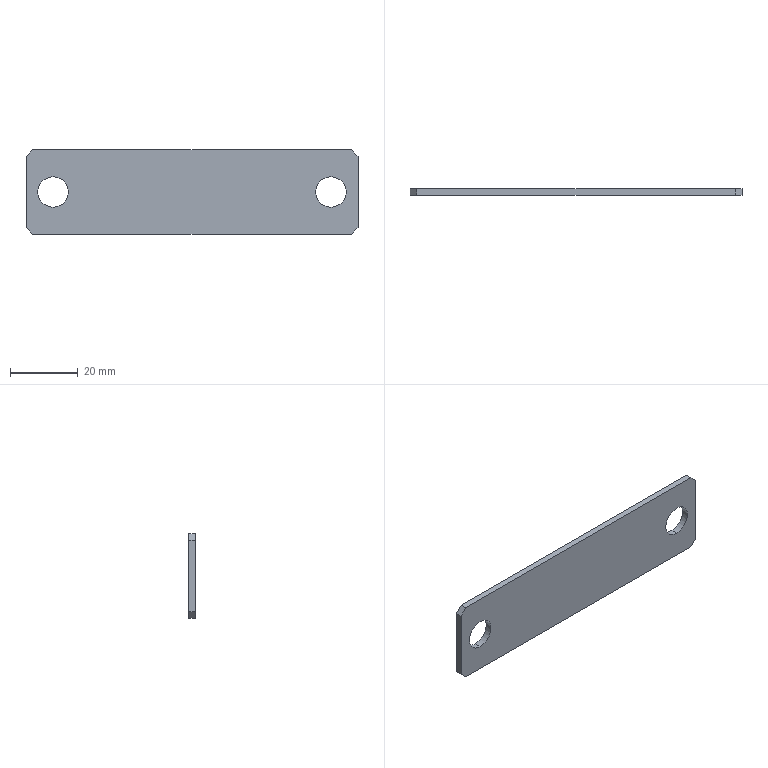Part | STEP file | Vibration plate 3-07_default | 1 solid | 14 faces | box 98 x 2 x 25 mm | volume 4630 mm3 | plane 10 | cylinder 4 | commonest cylinder face diameters 9 x4
STEP:
#1=CARTESIAN_POINT('',(0.,0.,0.));
#2=DIRECTION('',(0.,0.,1.));
#3=DIRECTION('',(1.,0.,0.));
#4=AXIS2_PLACEMENT_3D('',#1,#2,#3);
#5=CARTESIAN_POINT('',(41.,0.,4.5));
#6=VERTEX_POINT('',#5);
#7=CARTESIAN_POINT('',(41.,2.,4.5));
#8=VERTEX_POINT('',#7);
#9=CARTESIAN_POINT('',(41.,2.,4.5));
#10=DIRECTION('',(0.,1.,0.));
#11=VECTOR('',#10,1.);
#12=LINE('',#9,#11);
#13=CARTESIAN_POINT('',(41.,2.,0.));
#14=DIRECTION('',(0.,1.,0.));
#15=DIRECTION('',(0.,0.,1.));
#16=AXIS2_PLACEMENT_3D('',#13,#14,#15);
#17=CYLINDRICAL_SURFACE('',#16,4.5);
#18=CARTESIAN_POINT('',(6.283,0.));
#19=DIRECTION('',(0.,1.));
#20=VECTOR('',#19,1.);
#21=LINE('',#18,#20);
#22=(GEOMETRIC_REPRESENTATION_CONTEXT(2)PARAMETRIC_REPRESENTATION_CONTEXT()REPRESENTATION_CONTEXT('',''));
#23=DEFINITIONAL_REPRESENTATION('',(#21),#22);
#24=PCURVE('',#17,#23);
#25=CARTESIAN_POINT('',(41.,2.,0.));
#26=DIRECTION('',(0.,1.,0.));
#27=DIRECTION('',(0.,0.,1.));
#28=AXIS2_PLACEMENT_3D('',#25,#26,#27);
#29=CYLINDRICAL_SURFACE('',#28,4.5);
#30=CARTESIAN_POINT('',(0.,0.));
#31=DIRECTION('',(0.,1.));
#32=VECTOR('',#31,1.);
#33=LINE('',#30,#32);
#34=(GEOMETRIC_REPRESENTATION_CONTEXT(2)PARAMETRIC_REPRESENTATION_CONTEXT()REPRESENTATION_CONTEXT('',''));
#35=DEFINITIONAL_REPRESENTATION('',(#33),#34);
#36=PCURVE('',#29,#35);
#37=SURFACE_CURVE('',#12,(#24,#36),.PCURVE_S1.);
#38=EDGE_CURVE('',#6,#8,#37,.T.);
#39=ORIENTED_EDGE('',*,*,#38,.T.);
#40=CARTESIAN_POINT('',(41.,2.,-4.5));
#41=VERTEX_POINT('',#40);
#42=CARTESIAN_POINT('',(41.,2.,0.));
#43=DIRECTION('',(0.,-1.,0.));
#44=DIRECTION('',(0.,0.,1.));
#45=AXIS2_PLACEMENT_3D('',#42,#43,#44);
#46=CIRCLE('',#45,4.5);
#47=CARTESIAN_POINT('',(6.283,0.));
#48=DIRECTION('',(-1.,0.));
#49=VECTOR('',#48,1.);
#50=LINE('',#47,#49);
#51=(GEOMETRIC_REPRESENTATION_CONTEXT(2)PARAMETRIC_REPRESENTATION_CONTEXT()REPRESENTATION_CONTEXT('',''));
#52=DEFINITIONAL_REPRESENTATION('',(#50),#51);
#53=PCURVE('',#17,#52);
#54=CARTESIAN_POINT('',(0.,2.,0.));
#55=DIRECTION('',(0.,1.,0.));
#56=DIRECTION('',(0.,0.,1.));
#57=AXIS2_PLACEMENT_3D('',#54,#55,#56);
#58=PLANE('',#57);
#59=CARTESIAN_POINT('',(4.5,41.));
#60=CARTESIAN_POINT('',(4.5,33.206));
#61=CARTESIAN_POINT('',(-2.25,37.103));
#62=CARTESIAN_POINT('',(-9.,41.));
#63=CARTESIAN_POINT('',(-2.25,44.897));
#64=CARTESIAN_POINT('',(4.5,48.794));
#65=CARTESIAN_POINT('',(4.5,41.));
#66=(BOUNDED_CURVE()B_SPLINE_CURVE(2,(#59,#60,#61,#62,#63,#64,#65),.UNSPECIFIED.,.T.,.F.)B_SPLINE_CURVE_WITH_KNOTS((1,2,2,2,2,1),(-2.094,0.,2.094,4.189,6.283,8.378),.UNSPECIFIED.)CURVE()GEOMETRIC_REPRESENTATION_ITEM()RATIONAL_B_SPLINE_CURVE((1.,0.5,1.,0.5,1.,0.5,1.))REPRESENTATION_ITEM(''));
#67=(GEOMETRIC_REPRESENTATION_CONTEXT(2)PARAMETRIC_REPRESENTATION_CONTEXT()REPRESENTATION_CONTEXT('',''));
#68=DEFINITIONAL_REPRESENTATION('',(#66),#67);
#69=PCURVE('',#58,#68);
#70=SURFACE_CURVE('',#46,(#53,#69),.PCURVE_S1.);
#71=EDGE_CURVE('',#8,#41,#70,.T.);
#72=ORIENTED_EDGE('',*,*,#71,.T.);
#73=CARTESIAN_POINT('',(41.,0.,-4.5));
#74=VERTEX_POINT('',#73);
#75=CARTESIAN_POINT('',(41.,2.,-4.5));
#76=DIRECTION('',(0.,1.,0.));
#77=VECTOR('',#76,1.);
#78=LINE('',#75,#77);
#79=CARTESIAN_POINT('',(3.142,0.));
#80=DIRECTION('',(0.,1.));
#81=VECTOR('',#80,1.);
#82=LINE('',#79,#81);
#83=(GEOMETRIC_REPRESENTATION_CONTEXT(2)PARAMETRIC_REPRESENTATION_CONTEXT()REPRESENTATION_CONTEXT('',''));
#84=DEFINITIONAL_REPRESENTATION('',(#82),#83);
#85=PCURVE('',#17,#84);
#86=CARTESIAN_POINT('',(3.142,0.));
#87=DIRECTION('',(0.,1.));
#88=VECTOR('',#87,1.);
#89=LINE('',#86,#88);
#90=(GEOMETRIC_REPRESENTATION_CONTEXT(2)PARAMETRIC_REPRESENTATION_CONTEXT()REPRESENTATION_CONTEXT('',''));
#91=DEFINITIONAL_REPRESENTATION('',(#89),#90);
#92=PCURVE('',#29,#91);
#93=SURFACE_CURVE('',#78,(#85,#92),.PCURVE_S1.);
#94=EDGE_CURVE('',#74,#41,#93,.T.);
#95=ORIENTED_EDGE('',*,*,#94,.F.);
#96=CARTESIAN_POINT('',(41.,0.,0.));
#97=DIRECTION('',(0.,-1.,0.));
#98=DIRECTION('',(0.,0.,1.));
#99=AXIS2_PLACEMENT_3D('',#96,#97,#98);
#100=CIRCLE('',#99,4.5);
#101=CARTESIAN_POINT('',(6.283,-2.));
#102=DIRECTION('',(-1.,0.));
#103=VECTOR('',#102,1.);
#104=LINE('',#101,#103);
#105=(GEOMETRIC_REPRESENTATION_CONTEXT(2)PARAMETRIC_REPRESENTATION_CONTEXT()REPRESENTATION_CONTEXT('',''));
#106=DEFINITIONAL_REPRESENTATION('',(#104),#105);
#107=PCURVE('',#17,#106);
#108=CARTESIAN_POINT('',(0.,0.,0.));
#109=DIRECTION('',(0.,1.,0.));
#110=DIRECTION('',(0.,0.,1.));
#111=AXIS2_PLACEMENT_3D('',#108,#109,#110);
#112=PLANE('',#111);
#113=CARTESIAN_POINT('',(4.5,41.));
#114=CARTESIAN_POINT('',(4.5,33.206));
#115=CARTESIAN_POINT('',(-2.25,37.103));
#116=CARTESIAN_POINT('',(-9.,41.));
#117=CARTESIAN_POINT('',(-2.25,44.897));
#118=CARTESIAN_POINT('',(4.5,48.794));
#119=CARTESIAN_POINT('',(4.5,41.));
#120=(BOUNDED_CURVE()B_SPLINE_CURVE(2,(#113,#114,#115,#116,#117,#118,#119),.UNSPECIFIED.,.T.,.F.)B_SPLINE_CURVE_WITH_KNOTS((1,2,2,2,2,1),(-2.094,0.,2.094,4.189,6.283,8.378),.UNSPECIFIED.)CURVE()GEOMETRIC_REPRESENTATION_ITEM()RATIONAL_B_SPLINE_CURVE((1.,0.5,1.,0.5,1.,0.5,1.))REPRESENTATION_ITEM(''));
#121=(GEOMETRIC_REPRESENTATION_CONTEXT(2)PARAMETRIC_REPRESENTATION_CONTEXT()REPRESENTATION_CONTEXT('',''));
#122=DEFINITIONAL_REPRESENTATION('',(#120),#121);
#123=PCURVE('',#112,#122);
#124=SURFACE_CURVE('',#100,(#107,#123),.PCURVE_S1.);
#125=EDGE_CURVE('',#6,#74,#124,.T.);
#126=ORIENTED_EDGE('',*,*,#125,.F.);
#127=EDGE_LOOP('',(#39,#72,#95,#126));
#128=FACE_BOUND('',#127,.F.);
#129=ADVANCED_FACE('',(#128),#17,.F.);
#130=CARTESIAN_POINT('',(-41.,0.,4.5));
#131=VERTEX_POINT('',#130);
#132=CARTESIAN_POINT('',(-41.,2.,4.5));
#133=VERTEX_POINT('',#132);
#134=CARTESIAN_POINT('',(-41.,2.,4.5));
#135=DIRECTION('',(0.,1.,0.));
#136=VECTOR('',#135,1.);
#137=LINE('',#134,#136);
#138=CARTESIAN_POINT('',(-41.,2.,0.));
#139=DIRECTION('',(0.,1.,0.));
#140=DIRECTION('',(0.,0.,1.));
#141=AXIS2_PLACEMENT_3D('',#138,#139,#140);
#142=CYLINDRICAL_SURFACE('',#141,4.5);
#143=CARTESIAN_POINT('',(6.283,0.));
#144=DIRECTION('',(0.,1.));
#145=VECTOR('',#144,1.);
#146=LINE('',#143,#145);
#147=(GEOMETRIC_REPRESENTATION_CONTEXT(2)PARAMETRIC_REPRESENTATION_CONTEXT()REPRESENTATION_CONTEXT('',''));
#148=DEFINITIONAL_REPRESENTATION('',(#146),#147);
#149=PCURVE('',#142,#148);
#150=CARTESIAN_POINT('',(-41.,2.,0.));
#151=DIRECTION('',(0.,1.,0.));
#152=DIRECTION('',(0.,0.,1.));
#153=AXIS2_PLACEMENT_3D('',#150,#151,#152);
#154=CYLINDRICAL_SURFACE('',#153,4.5);
#155=CARTESIAN_POINT('',(0.,0.));
#156=DIRECTION('',(0.,1.));
#157=VECTOR('',#156,1.);
#158=LINE('',#155,#157);
#159=(GEOMETRIC_REPRESENTATION_CONTEXT(2)PARAMETRIC_REPRESENTATION_CONTEXT()REPRESENTATION_CONTEXT('',''));
#160=DEFINITIONAL_REPRESENTATION('',(#158),#159);
#161=PCURVE('',#154,#160);
#162=SURFACE_CURVE('',#137,(#149,#161),.PCURVE_S1.);
#163=EDGE_CURVE('',#131,#133,#162,.T.);
#164=ORIENTED_EDGE('',*,*,#163,.T.);
#165=CARTESIAN_POINT('',(-41.,2.,-4.5));
#166=VERTEX_POINT('',#165);
#167=CARTESIAN_POINT('',(-41.,2.,0.));
#168=DIRECTION('',(0.,-1.,0.));
#169=DIRECTION('',(0.,0.,1.));
#170=AXIS2_PLACEMENT_3D('',#167,#168,#169);
#171=CIRCLE('',#170,4.5);
#172=CARTESIAN_POINT('',(6.283,0.));
#173=DIRECTION('',(-1.,0.));
#174=VECTOR('',#173,1.);
#175=LINE('',#172,#174);
#176=(GEOMETRIC_REPRESENTATION_CONTEXT(2)PARAMETRIC_REPRESENTATION_CONTEXT()REPRESENTATION_CONTEXT('',''));
#177=DEFINITIONAL_REPRESENTATION('',(#175),#176);
#178=PCURVE('',#142,#177);
#179=CARTESIAN_POINT('',(4.5,-41.));
#180=CARTESIAN_POINT('',(4.5,-48.794));
#181=CARTESIAN_POINT('',(-2.25,-44.897));
#182=CARTESIAN_POINT('',(-9.,-41.));
#183=CARTESIAN_POINT('',(-2.25,-37.103));
#184=CARTESIAN_POINT('',(4.5,-33.206));
#185=CARTESIAN_POINT('',(4.5,-41.));
#186=(BOUNDED_CURVE()B_SPLINE_CURVE(2,(#179,#180,#181,#182,#183,#184,#185),.UNSPECIFIED.,.T.,.F.)B_SPLINE_CURVE_WITH_KNOTS((1,2,2,2,2,1),(-2.094,0.,2.094,4.189,6.283,8.378),.UNSPECIFIED.)CURVE()GEOMETRIC_REPRESENTATION_ITEM()RATIONAL_B_SPLINE_CURVE((1.,0.5,1.,0.5,1.,0.5,1.))REPRESENTATION_ITEM(''));
#187=(GEOMETRIC_REPRESENTATION_CONTEXT(2)PARAMETRIC_REPRESENTATION_CONTEXT()REPRESENTATION_CONTEXT('',''));
#188=DEFINITIONAL_REPRESENTATION('',(#186),#187);
#189=PCURVE('',#58,#188);
#190=SURFACE_CURVE('',#171,(#178,#189),.PCURVE_S1.);
#191=EDGE_CURVE('',#133,#166,#190,.T.);
#192=ORIENTED_EDGE('',*,*,#191,.T.);
#193=CARTESIAN_POINT('',(-41.,0.,-4.5));
#194=VERTEX_POINT('',#193);
#195=CARTESIAN_POINT('',(-41.,2.,-4.5));
#196=DIRECTION('',(0.,1.,0.));
#197=VECTOR('',#196,1.);
#198=LINE('',#195,#197);
#199=CARTESIAN_POINT('',(3.142,0.));
#200=DIRECTION('',(0.,1.));
#201=VECTOR('',#200,1.);
#202=LINE('',#199,#201);
#203=(GEOMETRIC_REPRESENTATION_CONTEXT(2)PARAMETRIC_REPRESENTATION_CONTEXT()REPRESENTATION_CONTEXT('',''));
#204=DEFINITIONAL_REPRESENTATION('',(#202),#203);
#205=PCURVE('',#142,#204);
#206=CARTESIAN_POINT('',(3.142,0.));
#207=DIRECTION('',(0.,1.));
#208=VECTOR('',#207,1.);
#209=LINE('',#206,#208);
#210=(GEOMETRIC_REPRESENTATION_CONTEXT(2)PARAMETRIC_REPRESENTATION_CONTEXT()REPRESENTATION_CONTEXT('',''));
#211=DEFINITIONAL_REPRESENTATION('',(#209),#210);
#212=PCURVE('',#154,#211);
#213=SURFACE_CURVE('',#198,(#205,#212),.PCURVE_S1.);
#214=EDGE_CURVE('',#194,#166,#213,.T.);
#215=ORIENTED_EDGE('',*,*,#214,.F.);
#216=CARTESIAN_POINT('',(-41.,0.,0.));
#217=DIRECTION('',(0.,-1.,0.));
#218=DIRECTION('',(0.,0.,1.));
#219=AXIS2_PLACEMENT_3D('',#216,#217,#218);
#220=CIRCLE('',#219,4.5);
#221=CARTESIAN_POINT('',(6.283,-2.));
#222=DIRECTION('',(-1.,0.));
#223=VECTOR('',#222,1.);
#224=LINE('',#221,#223);
#225=(GEOMETRIC_REPRESENTATION_CONTEXT(2)PARAMETRIC_REPRESENTATION_CONTEXT()REPRESENTATION_CONTEXT('',''));
#226=DEFINITIONAL_REPRESENTATION('',(#224),#225);
#227=PCURVE('',#142,#226);
#228=CARTESIAN_POINT('',(4.5,-41.));
#229=CARTESIAN_POINT('',(4.5,-48.794));
#230=CARTESIAN_POINT('',(-2.25,-44.897));
#231=CARTESIAN_POINT('',(-9.,-41.));
#232=CARTESIAN_POINT('',(-2.25,-37.103));
#233=CARTESIAN_POINT('',(4.5,-33.206));
#234=CARTESIAN_POINT('',(4.5,-41.));
#235=(BOUNDED_CURVE()B_SPLINE_CURVE(2,(#228,#229,#230,#231,#232,#233,#234),.UNSPECIFIED.,.T.,.F.)B_SPLINE_CURVE_WITH_KNOTS((1,2,2,2,2,1),(-2.094,0.,2.094,4.189,6.283,8.378),.UNSPECIFIED.)CURVE()GEOMETRIC_REPRESENTATION_ITEM()RATIONAL_B_SPLINE_CURVE((1.,0.5,1.,0.5,1.,0.5,1.))REPRESENTATION_ITEM(''));
#236=(GEOMETRIC_REPRESENTATION_CONTEXT(2)PARAMETRIC_REPRESENTATION_CONTEXT()REPRESENTATION_CONTEXT('',''));
#237=DEFINITIONAL_REPRESENTATION('',(#235),#236);
#238=PCURVE('',#112,#237);
#239=SURFACE_CURVE('',#220,(#227,#238),.PCURVE_S1.);
#240=EDGE_CURVE('',#131,#194,#239,.T.);
#241=ORIENTED_EDGE('',*,*,#240,.F.);
#242=EDGE_LOOP('',(#164,#192,#215,#241));
#243=FACE_BOUND('',#242,.F.);
#244=ADVANCED_FACE('',(#243),#142,.F.);
#245=ORIENTED_EDGE('',*,*,#125,.F.);
#246=CARTESIAN_POINT('',(41.,0.,0.));
#247=DIRECTION('',(0.,-1.,0.));
#248=DIRECTION('',(0.,0.,1.));
#249=AXIS2_PLACEMENT_3D('',#246,#247,#248);
#250=CIRCLE('',#249,4.5);
#251=CARTESIAN_POINT('',(4.5,41.));
#252=CARTESIAN_POINT('',(4.5,33.206));
#253=CARTESIAN_POINT('',(-2.25,37.103));
#254=CARTESIAN_POINT('',(-9.,41.));
#255=CARTESIAN_POINT('',(-2.25,44.897));
#256=CARTESIAN_POINT('',(4.5,48.794));
#257=CARTESIAN_POINT('',(4.5,41.));
#258=(BOUNDED_CURVE()B_SPLINE_CURVE(2,(#251,#252,#253,#254,#255,#256,#257),.UNSPECIFIED.,.T.,.F.)B_SPLINE_CURVE_WITH_KNOTS((1,2,2,2,2,1),(-2.094,0.,2.094,4.189,6.283,8.378),.UNSPECIFIED.)CURVE()GEOMETRIC_REPRESENTATION_ITEM()RATIONAL_B_SPLINE_CURVE((1.,0.5,1.,0.5,1.,0.5,1.))REPRESENTATION_ITEM(''));
#259=(GEOMETRIC_REPRESENTATION_CONTEXT(2)PARAMETRIC_REPRESENTATION_CONTEXT()REPRESENTATION_CONTEXT('',''));
#260=DEFINITIONAL_REPRESENTATION('',(#258),#259);
#261=PCURVE('',#112,#260);
#262=CARTESIAN_POINT('',(6.283,-2.));
#263=DIRECTION('',(-1.,0.));
#264=VECTOR('',#263,1.);
#265=LINE('',#262,#264);
#266=(GEOMETRIC_REPRESENTATION_CONTEXT(2)PARAMETRIC_REPRESENTATION_CONTEXT()REPRESENTATION_CONTEXT('',''));
#267=DEFINITIONAL_REPRESENTATION('',(#265),#266);
#268=PCURVE('',#29,#267);
#269=SURFACE_CURVE('',#250,(#261,#268),.PCURVE_S1.);
#270=EDGE_CURVE('',#74,#6,#269,.T.);
#271=ORIENTED_EDGE('',*,*,#270,.F.);
#272=EDGE_LOOP('',(#245,#271));
#273=FACE_BOUND('',#272,.T.);
#274=ORIENTED_EDGE('',*,*,#240,.F.);
#275=CARTESIAN_POINT('',(-41.,0.,0.));
#276=DIRECTION('',(0.,-1.,0.));
#277=DIRECTION('',(0.,0.,1.));
#278=AXIS2_PLACEMENT_3D('',#275,#276,#277);
#279=CIRCLE('',#278,4.5);
#280=CARTESIAN_POINT('',(4.5,-41.));
#281=CARTESIAN_POINT('',(4.5,-48.794));
#282=CARTESIAN_POINT('',(-2.25,-44.897));
#283=CARTESIAN_POINT('',(-9.,-41.));
#284=CARTESIAN_POINT('',(-2.25,-37.103));
#285=CARTESIAN_POINT('',(4.5,-33.206));
#286=CARTESIAN_POINT('',(4.5,-41.));
#287=(BOUNDED_CURVE()B_SPLINE_CURVE(2,(#280,#281,#282,#283,#284,#285,#286),.UNSPECIFIED.,.T.,.F.)B_SPLINE_CURVE_WITH_KNOTS((1,2,2,2,2,1),(-2.094,0.,2.094,4.189,6.283,8.378),.UNSPECIFIED.)CURVE()GEOMETRIC_REPRESENTATION_ITEM()RATIONAL_B_SPLINE_CURVE((1.,0.5,1.,0.5,1.,0.5,1.))REPRESENTATION_ITEM(''));
#288=(GEOMETRIC_REPRESENTATION_CONTEXT(2)PARAMETRIC_REPRESENTATION_CONTEXT()REPRESENTATION_CONTEXT('',''));
#289=DEFINITIONAL_REPRESENTATION('',(#287),#288);
#290=PCURVE('',#112,#289);
#291=CARTESIAN_POINT('',(6.283,-2.));
#292=DIRECTION('',(-1.,0.));
#293=VECTOR('',#292,1.);
#294=LINE('',#291,#293);
#295=(GEOMETRIC_REPRESENTATION_CONTEXT(2)PARAMETRIC_REPRESENTATION_CONTEXT()REPRESENTATION_CONTEXT('',''));
#296=DEFINITIONAL_REPRESENTATION('',(#294),#295);
#297=PCURVE('',#154,#296);
#298=SURFACE_CURVE('',#279,(#290,#297),.PCURVE_S1.);
#299=EDGE_CURVE('',#194,#131,#298,.T.);
#300=ORIENTED_EDGE('',*,*,#299,.F.);
#301=EDGE_LOOP('',(#274,#300));
#302=FACE_BOUND('',#301,.T.);
#303=CARTESIAN_POINT('',(-49.,0.,10.5));
#304=VERTEX_POINT('',#303);
#305=CARTESIAN_POINT('',(-47.,0.,12.5));
#306=VERTEX_POINT('',#305);
#307=CARTESIAN_POINT('',(-49.,0.,10.5));
#308=DIRECTION('',(0.7071,0.,0.7071));
#309=VECTOR('',#308,1.);
#310=LINE('',#307,#309);
#311=CARTESIAN_POINT('',(10.5,-49.));
#312=DIRECTION('',(0.7071,0.7071));
#313=VECTOR('',#312,1.);
#314=LINE('',#311,#313);
#315=(GEOMETRIC_REPRESENTATION_CONTEXT(2)PARAMETRIC_REPRESENTATION_CONTEXT()REPRESENTATION_CONTEXT('',''));
#316=DEFINITIONAL_REPRESENTATION('',(#314),#315);
#317=PCURVE('',#112,#316);
#318=CARTESIAN_POINT('',(-48.,1.,11.5));
#319=DIRECTION('',(-0.7071,0.,0.7071));
#320=DIRECTION('',(0.7071,0.,0.7071));
#321=AXIS2_PLACEMENT_3D('',#318,#319,#320);
#322=PLANE('',#321);
#323=CARTESIAN_POINT('',(-1.414,-1.));
#324=DIRECTION('',(1.,0.));
#325=VECTOR('',#324,1.);
#326=LINE('',#323,#325);
#327=(GEOMETRIC_REPRESENTATION_CONTEXT(2)PARAMETRIC_REPRESENTATION_CONTEXT()REPRESENTATION_CONTEXT('',''));
#328=DEFINITIONAL_REPRESENTATION('',(#326),#327);
#329=PCURVE('',#322,#328);
#330=SURFACE_CURVE('',#310,(#317,#329),.PCURVE_S1.);
#331=EDGE_CURVE('',#304,#306,#330,.T.);
#332=ORIENTED_EDGE('',*,*,#331,.F.);
#333=CARTESIAN_POINT('',(-49.,0.,-10.5));
#334=VERTEX_POINT('',#333);
#335=CARTESIAN_POINT('',(-49.,0.,0.));
#336=DIRECTION('',(0.,0.,1.));
#337=VECTOR('',#336,1.);
#338=LINE('',#335,#337);
#339=CARTESIAN_POINT('',(0.,-49.));
#340=DIRECTION('',(1.,0.));
#341=VECTOR('',#340,1.);
#342=LINE('',#339,#341);
#343=(GEOMETRIC_REPRESENTATION_CONTEXT(2)PARAMETRIC_REPRESENTATION_CONTEXT()REPRESENTATION_CONTEXT('',''));
#344=DEFINITIONAL_REPRESENTATION('',(#342),#343);
#345=PCURVE('',#112,#344);
#346=CARTESIAN_POINT('',(-49.,0.,-12.5));
#347=DIRECTION('',(-1.,0.,0.));
#348=DIRECTION('',(0.,0.,1.));
#349=AXIS2_PLACEMENT_3D('',#346,#347,#348);
#350=PLANE('',#349);
#351=CARTESIAN_POINT('',(12.5,0.));
#352=DIRECTION('',(1.,0.));
#353=VECTOR('',#352,1.);
#354=LINE('',#351,#353);
#355=(GEOMETRIC_REPRESENTATION_CONTEXT(2)PARAMETRIC_REPRESENTATION_CONTEXT()REPRESENTATION_CONTEXT('',''));
#356=DEFINITIONAL_REPRESENTATION('',(#354),#355);
#357=PCURVE('',#350,#356);
#358=SURFACE_CURVE('',#338,(#345,#357),.PCURVE_S1.);
#359=EDGE_CURVE('',#334,#304,#358,.T.);
#360=ORIENTED_EDGE('',*,*,#359,.F.);
#361=CARTESIAN_POINT('',(-47.,0.,-12.5));
#362=VERTEX_POINT('',#361);
#363=CARTESIAN_POINT('',(-47.,0.,-12.5));
#364=DIRECTION('',(-0.7071,0.,0.7071));
#365=VECTOR('',#364,1.);
#366=LINE('',#363,#365);
#367=CARTESIAN_POINT('',(-12.5,-47.));
#368=DIRECTION('',(0.7071,-0.7071));
#369=VECTOR('',#368,1.);
#370=LINE('',#367,#369);
#371=(GEOMETRIC_REPRESENTATION_CONTEXT(2)PARAMETRIC_REPRESENTATION_CONTEXT()REPRESENTATION_CONTEXT('',''));
#372=DEFINITIONAL_REPRESENTATION('',(#370),#371);
#373=PCURVE('',#112,#372);
#374=CARTESIAN_POINT('',(-48.,1.,-11.5));
#375=DIRECTION('',(-0.7071,0.,-0.7071));
#376=DIRECTION('',(-0.7071,0.,0.7071));
#377=AXIS2_PLACEMENT_3D('',#374,#375,#376);
#378=PLANE('',#377);
#379=CARTESIAN_POINT('',(-1.414,-1.));
#380=DIRECTION('',(1.,0.));
#381=VECTOR('',#380,1.);
#382=LINE('',#379,#381);
#383=(GEOMETRIC_REPRESENTATION_CONTEXT(2)PARAMETRIC_REPRESENTATION_CONTEXT()REPRESENTATION_CONTEXT('',''));
#384=DEFINITIONAL_REPRESENTATION('',(#382),#383);
#385=PCURVE('',#378,#384);
#386=SURFACE_CURVE('',#366,(#373,#385),.PCURVE_S1.);
#387=EDGE_CURVE('',#362,#334,#386,.T.);
#388=ORIENTED_EDGE('',*,*,#387,.F.);
#389=CARTESIAN_POINT('',(47.,0.,-12.5));
#390=VERTEX_POINT('',#389);
#391=CARTESIAN_POINT('',(0.,0.,-12.5));
#392=DIRECTION('',(-1.,0.,0.));
#393=VECTOR('',#392,1.);
#394=LINE('',#391,#393);
#395=CARTESIAN_POINT('',(-12.5,0.));
#396=DIRECTION('',(0.,-1.));
#397=VECTOR('',#396,1.);
#398=LINE('',#395,#397);
#399=(GEOMETRIC_REPRESENTATION_CONTEXT(2)PARAMETRIC_REPRESENTATION_CONTEXT()REPRESENTATION_CONTEXT('',''));
#400=DEFINITIONAL_REPRESENTATION('',(#398),#399);
#401=PCURVE('',#112,#400);
#402=CARTESIAN_POINT('',(49.,0.,-12.5));
#403=DIRECTION('',(0.,0.,-1.));
#404=DIRECTION('',(-1.,0.,0.));
#405=AXIS2_PLACEMENT_3D('',#402,#403,#404);
#406=PLANE('',#405);
#407=CARTESIAN_POINT('',(49.,0.));
#408=DIRECTION('',(1.,0.));
#409=VECTOR('',#408,1.);
#410=LINE('',#407,#409);
#411=(GEOMETRIC_REPRESENTATION_CONTEXT(2)PARAMETRIC_REPRESENTATION_CONTEXT()REPRESENTATION_CONTEXT('',''));
#412=DEFINITIONAL_REPRESENTATION('',(#410),#411);
#413=PCURVE('',#406,#412);
#414=SURFACE_CURVE('',#394,(#401,#413),.PCURVE_S1.);
#415=EDGE_CURVE('',#390,#362,#414,.T.);
#416=ORIENTED_EDGE('',*,*,#415,.F.);
#417=CARTESIAN_POINT('',(49.,0.,-10.5));
#418=VERTEX_POINT('',#417);
#419=CARTESIAN_POINT('',(49.,0.,-10.5));
#420=DIRECTION('',(-0.7071,0.,-0.7071));
#421=VECTOR('',#420,1.);
#422=LINE('',#419,#421);
#423=CARTESIAN_POINT('',(-10.5,49.));
#424=DIRECTION('',(-0.7071,-0.7071));
#425=VECTOR('',#424,1.);
#426=LINE('',#423,#425);
#427=(GEOMETRIC_REPRESENTATION_CONTEXT(2)PARAMETRIC_REPRESENTATION_CONTEXT()REPRESENTATION_CONTEXT('',''));
#428=DEFINITIONAL_REPRESENTATION('',(#426),#427);
#429=PCURVE('',#112,#428);
#430=CARTESIAN_POINT('',(48.,1.,-11.5));
#431=DIRECTION('',(0.7071,0.,-0.7071));
#432=DIRECTION('',(-0.7071,0.,-0.7071));
#433=AXIS2_PLACEMENT_3D('',#430,#431,#432);
#434=PLANE('',#433);
#435=CARTESIAN_POINT('',(-1.414,-1.));
#436=DIRECTION('',(1.,0.));
#437=VECTOR('',#436,1.);
#438=LINE('',#435,#437);
#439=(GEOMETRIC_REPRESENTATION_CONTEXT(2)PARAMETRIC_REPRESENTATION_CONTEXT()REPRESENTATION_CONTEXT('',''));
#440=DEFINITIONAL_REPRESENTATION('',(#438),#439);
#441=PCURVE('',#434,#440);
#442=SURFACE_CURVE('',#422,(#429,#441),.PCURVE_S1.);
#443=EDGE_CURVE('',#418,#390,#442,.T.);
#444=ORIENTED_EDGE('',*,*,#443,.F.);
#445=CARTESIAN_POINT('',(49.,0.,10.5));
#446=VERTEX_POINT('',#445);
#447=CARTESIAN_POINT('',(49.,0.,0.));
#448=DIRECTION('',(0.,0.,-1.));
#449=VECTOR('',#448,1.);
#450=LINE('',#447,#449);
#451=CARTESIAN_POINT('',(0.,49.));
#452=DIRECTION('',(-1.,0.));
#453=VECTOR('',#452,1.);
#454=LINE('',#451,#453);
#455=(GEOMETRIC_REPRESENTATION_CONTEXT(2)PARAMETRIC_REPRESENTATION_CONTEXT()REPRESENTATION_CONTEXT('',''));
#456=DEFINITIONAL_REPRESENTATION('',(#454),#455);
#457=PCURVE('',#112,#456);
#458=CARTESIAN_POINT('',(49.,0.,12.5));
#459=DIRECTION('',(1.,0.,0.));
#460=DIRECTION('',(0.,0.,-1.));
#461=AXIS2_PLACEMENT_3D('',#458,#459,#460);
#462=PLANE('',#461);
#463=CARTESIAN_POINT('',(12.5,0.));
#464=DIRECTION('',(1.,0.));
#465=VECTOR('',#464,1.);
#466=LINE('',#463,#465);
#467=(GEOMETRIC_REPRESENTATION_CONTEXT(2)PARAMETRIC_REPRESENTATION_CONTEXT()REPRESENTATION_CONTEXT('',''));
#468=DEFINITIONAL_REPRESENTATION('',(#466),#467);
#469=PCURVE('',#462,#468);
#470=SURFACE_CURVE('',#450,(#457,#469),.PCURVE_S1.);
#471=EDGE_CURVE('',#446,#418,#470,.T.);
#472=ORIENTED_EDGE('',*,*,#471,.F.);
#473=CARTESIAN_POINT('',(47.,0.,12.5));
#474=VERTEX_POINT('',#473);
#475=CARTESIAN_POINT('',(47.,0.,12.5));
#476=DIRECTION('',(0.7071,0.,-0.7071));
#477=VECTOR('',#476,1.);
#478=LINE('',#475,#477);
#479=CARTESIAN_POINT('',(12.5,47.));
#480=DIRECTION('',(-0.7071,0.7071));
#481=VECTOR('',#480,1.);
#482=LINE('',#479,#481);
#483=(GEOMETRIC_REPRESENTATION_CONTEXT(2)PARAMETRIC_REPRESENTATION_CONTEXT()REPRESENTATION_CONTEXT('',''));
#484=DEFINITIONAL_REPRESENTATION('',(#482),#483);
#485=PCURVE('',#112,#484);
#486=CARTESIAN_POINT('',(48.,1.,11.5));
#487=DIRECTION('',(0.7071,0.,0.7071));
#488=DIRECTION('',(0.7071,0.,-0.7071));
#489=AXIS2_PLACEMENT_3D('',#486,#487,#488);
#490=PLANE('',#489);
#491=CARTESIAN_POINT('',(-1.414,-1.));
#492=DIRECTION('',(1.,0.));
#493=VECTOR('',#492,1.);
#494=LINE('',#491,#493);
#495=(GEOMETRIC_REPRESENTATION_CONTEXT(2)PARAMETRIC_REPRESENTATION_CONTEXT()REPRESENTATION_CONTEXT('',''));
#496=DEFINITIONAL_REPRESENTATION('',(#494),#495);
#497=PCURVE('',#490,#496);
#498=SURFACE_CURVE('',#478,(#485,#497),.PCURVE_S1.);
#499=EDGE_CURVE('',#474,#446,#498,.T.);
#500=ORIENTED_EDGE('',*,*,#499,.F.);
#501=CARTESIAN_POINT('',(0.,0.,12.5));
#502=DIRECTION('',(1.,0.,0.));
#503=VECTOR('',#502,1.);
#504=LINE('',#501,#503);
#505=CARTESIAN_POINT('',(12.5,0.));
#506=DIRECTION('',(0.,1.));
#507=VECTOR('',#506,1.);
#508=LINE('',#505,#507);
#509=(GEOMETRIC_REPRESENTATION_CONTEXT(2)PARAMETRIC_REPRESENTATION_CONTEXT()REPRESENTATION_CONTEXT('',''));
#510=DEFINITIONAL_REPRESENTATION('',(#508),#509);
#511=PCURVE('',#112,#510);
#512=CARTESIAN_POINT('',(-49.,0.,12.5));
#513=DIRECTION('',(0.,0.,1.));
#514=DIRECTION('',(1.,0.,0.));
#515=AXIS2_PLACEMENT_3D('',#512,#513,#514);
#516=PLANE('',#515);
#517=CARTESIAN_POINT('',(49.,0.));
#518=DIRECTION('',(1.,0.));
#519=VECTOR('',#518,1.);
#520=LINE('',#517,#519);
#521=(GEOMETRIC_REPRESENTATION_CONTEXT(2)PARAMETRIC_REPRESENTATION_CONTEXT()REPRESENTATION_CONTEXT('',''));
#522=DEFINITIONAL_REPRESENTATION('',(#520),#521);
#523=PCURVE('',#516,#522);
#524=SURFACE_CURVE('',#504,(#511,#523),.PCURVE_S1.);
#525=EDGE_CURVE('',#306,#474,#524,.T.);
#526=ORIENTED_EDGE('',*,*,#525,.F.);
#527=EDGE_LOOP('',(#332,#360,#388,#416,#444,#472,#500,#526));
#528=FACE_BOUND('',#527,.T.);
#529=ADVANCED_FACE('',(#273,#302,#528),#112,.F.);
#530=CARTESIAN_POINT('',(41.,2.,0.));
#531=DIRECTION('',(0.,-1.,0.));
#532=DIRECTION('',(0.,0.,1.));
#533=AXIS2_PLACEMENT_3D('',#530,#531,#532);
#534=CIRCLE('',#533,4.5);
#535=CARTESIAN_POINT('',(6.283,0.));
#536=DIRECTION('',(-1.,0.));
#537=VECTOR('',#536,1.);
#538=LINE('',#535,#537);
#539=(GEOMETRIC_REPRESENTATION_CONTEXT(2)PARAMETRIC_REPRESENTATION_CONTEXT()REPRESENTATION_CONTEXT('',''));
#540=DEFINITIONAL_REPRESENTATION('',(#538),#539);
#541=PCURVE('',#29,#540);
#542=CARTESIAN_POINT('',(4.5,41.));
#543=CARTESIAN_POINT('',(4.5,33.206));
#544=CARTESIAN_POINT('',(-2.25,37.103));
#545=CARTESIAN_POINT('',(-9.,41.));
#546=CARTESIAN_POINT('',(-2.25,44.897));
#547=CARTESIAN_POINT('',(4.5,48.794));
#548=CARTESIAN_POINT('',(4.5,41.));
#549=(BOUNDED_CURVE()B_SPLINE_CURVE(2,(#542,#543,#544,#545,#546,#547,#548),.UNSPECIFIED.,.T.,.F.)B_SPLINE_CURVE_WITH_KNOTS((1,2,2,2,2,1),(-2.094,0.,2.094,4.189,6.283,8.378),.UNSPECIFIED.)CURVE()GEOMETRIC_REPRESENTATION_ITEM()RATIONAL_B_SPLINE_CURVE((1.,0.5,1.,0.5,1.,0.5,1.))REPRESENTATION_ITEM(''));
#550=(GEOMETRIC_REPRESENTATION_CONTEXT(2)PARAMETRIC_REPRESENTATION_CONTEXT()REPRESENTATION_CONTEXT('',''));
#551=DEFINITIONAL_REPRESENTATION('',(#549),#550);
#552=PCURVE('',#58,#551);
#553=SURFACE_CURVE('',#534,(#541,#552),.PCURVE_S1.);
#554=EDGE_CURVE('',#41,#8,#553,.T.);
#555=ORIENTED_EDGE('',*,*,#554,.T.);
#556=ORIENTED_EDGE('',*,*,#38,.F.);
#557=ORIENTED_EDGE('',*,*,#270,.F.);
#558=ORIENTED_EDGE('',*,*,#94,.T.);
#559=EDGE_LOOP('',(#555,#556,#557,#558));
#560=FACE_BOUND('',#559,.F.);
#561=ADVANCED_FACE('',(#560),#29,.F.);
#562=CARTESIAN_POINT('',(-41.,2.,0.));
#563=DIRECTION('',(0.,-1.,0.));
#564=DIRECTION('',(0.,0.,1.));
#565=AXIS2_PLACEMENT_3D('',#562,#563,#564);
#566=CIRCLE('',#565,4.5);
#567=CARTESIAN_POINT('',(6.283,0.));
#568=DIRECTION('',(-1.,0.));
#569=VECTOR('',#568,1.);
#570=LINE('',#567,#569);
#571=(GEOMETRIC_REPRESENTATION_CONTEXT(2)PARAMETRIC_REPRESENTATION_CONTEXT()REPRESENTATION_CONTEXT('',''));
#572=DEFINITIONAL_REPRESENTATION('',(#570),#571);
#573=PCURVE('',#154,#572);
#574=CARTESIAN_POINT('',(4.5,-41.));
#575=CARTESIAN_POINT('',(4.5,-48.794));
#576=CARTESIAN_POINT('',(-2.25,-44.897));
#577=CARTESIAN_POINT('',(-9.,-41.));
#578=CARTESIAN_POINT('',(-2.25,-37.103));
#579=CARTESIAN_POINT('',(4.5,-33.206));
#580=CARTESIAN_POINT('',(4.5,-41.));
#581=(BOUNDED_CURVE()B_SPLINE_CURVE(2,(#574,#575,#576,#577,#578,#579,#580),.UNSPECIFIED.,.T.,.F.)B_SPLINE_CURVE_WITH_KNOTS((1,2,2,2,2,1),(-2.094,0.,2.094,4.189,6.283,8.378),.UNSPECIFIED.)CURVE()GEOMETRIC_REPRESENTATION_ITEM()RATIONAL_B_SPLINE_CURVE((1.,0.5,1.,0.5,1.,0.5,1.))REPRESENTATION_ITEM(''));
#582=(GEOMETRIC_REPRESENTATION_CONTEXT(2)PARAMETRIC_REPRESENTATION_CONTEXT()REPRESENTATION_CONTEXT('',''));
#583=DEFINITIONAL_REPRESENTATION('',(#581),#582);
#584=PCURVE('',#58,#583);
#585=SURFACE_CURVE('',#566,(#573,#584),.PCURVE_S1.);
#586=EDGE_CURVE('',#166,#133,#585,.T.);
#587=ORIENTED_EDGE('',*,*,#586,.T.);
#588=ORIENTED_EDGE('',*,*,#163,.F.);
#589=ORIENTED_EDGE('',*,*,#299,.F.);
#590=ORIENTED_EDGE('',*,*,#214,.T.);
#591=EDGE_LOOP('',(#587,#588,#589,#590));
#592=FACE_BOUND('',#591,.F.);
#593=ADVANCED_FACE('',(#592),#154,.F.);
#594=ORIENTED_EDGE('',*,*,#525,.T.);
#595=CARTESIAN_POINT('',(47.,2.,12.5));
#596=VERTEX_POINT('',#595);
#597=CARTESIAN_POINT('',(47.,0.,12.5));
#598=DIRECTION('',(0.,1.,0.));
#599=VECTOR('',#598,1.);
#600=LINE('',#597,#599);
#601=CARTESIAN_POINT('',(96.,0.));
#602=DIRECTION('',(0.,1.));
#603=VECTOR('',#602,1.);
#604=LINE('',#601,#603);
#605=(GEOMETRIC_REPRESENTATION_CONTEXT(2)PARAMETRIC_REPRESENTATION_CONTEXT()REPRESENTATION_CONTEXT('',''));
#606=DEFINITIONAL_REPRESENTATION('',(#604),#605);
#607=PCURVE('',#516,#606);
#608=CARTESIAN_POINT('',(-1.414,-1.));
#609=DIRECTION('',(0.,1.));
#610=VECTOR('',#609,1.);
#611=LINE('',#608,#610);
#612=(GEOMETRIC_REPRESENTATION_CONTEXT(2)PARAMETRIC_REPRESENTATION_CONTEXT()REPRESENTATION_CONTEXT('',''));
#613=DEFINITIONAL_REPRESENTATION('',(#611),#612);
#614=PCURVE('',#490,#613);
#615=SURFACE_CURVE('',#600,(#607,#614),.PCURVE_S1.);
#616=EDGE_CURVE('',#474,#596,#615,.T.);
#617=ORIENTED_EDGE('',*,*,#616,.T.);
#618=CARTESIAN_POINT('',(-47.,2.,12.5));
#619=VERTEX_POINT('',#618);
#620=CARTESIAN_POINT('',(-49.,2.,12.5));
#621=DIRECTION('',(-1.,0.,0.));
#622=VECTOR('',#621,1.);
#623=LINE('',#620,#622);
#624=CARTESIAN_POINT('',(0.,2.));
#625=DIRECTION('',(-1.,0.));
#626=VECTOR('',#625,1.);
#627=LINE('',#624,#626);
#628=(GEOMETRIC_REPRESENTATION_CONTEXT(2)PARAMETRIC_REPRESENTATION_CONTEXT()REPRESENTATION_CONTEXT('',''));
#629=DEFINITIONAL_REPRESENTATION('',(#627),#628);
#630=PCURVE('',#516,#629);
#631=CARTESIAN_POINT('',(12.5,-49.));
#632=DIRECTION('',(0.,-1.));
#633=VECTOR('',#632,1.);
#634=LINE('',#631,#633);
#635=(GEOMETRIC_REPRESENTATION_CONTEXT(2)PARAMETRIC_REPRESENTATION_CONTEXT()REPRESENTATION_CONTEXT('',''));
#636=DEFINITIONAL_REPRESENTATION('',(#634),#635);
#637=PCURVE('',#58,#636);
#638=SURFACE_CURVE('',#623,(#630,#637),.PCURVE_S1.);
#639=EDGE_CURVE('',#596,#619,#638,.T.);
#640=ORIENTED_EDGE('',*,*,#639,.T.);
#641=CARTESIAN_POINT('',(-47.,0.,12.5));
#642=DIRECTION('',(0.,-1.,0.));
#643=VECTOR('',#642,1.);
#644=LINE('',#641,#643);
#645=CARTESIAN_POINT('',(2.,0.));
#646=DIRECTION('',(0.,-1.));
#647=VECTOR('',#646,1.);
#648=LINE('',#645,#647);
#649=(GEOMETRIC_REPRESENTATION_CONTEXT(2)PARAMETRIC_REPRESENTATION_CONTEXT()REPRESENTATION_CONTEXT('',''));
#650=DEFINITIONAL_REPRESENTATION('',(#648),#649);
#651=PCURVE('',#516,#650);
#652=CARTESIAN_POINT('',(1.414,-1.));
#653=DIRECTION('',(0.,-1.));
#654=VECTOR('',#653,1.);
#655=LINE('',#652,#654);
#656=(GEOMETRIC_REPRESENTATION_CONTEXT(2)PARAMETRIC_REPRESENTATION_CONTEXT()REPRESENTATION_CONTEXT('',''));
#657=DEFINITIONAL_REPRESENTATION('',(#655),#656);
#658=PCURVE('',#322,#657);
#659=SURFACE_CURVE('',#644,(#651,#658),.PCURVE_S1.);
#660=EDGE_CURVE('',#619,#306,#659,.T.);
#661=ORIENTED_EDGE('',*,*,#660,.T.);
#662=EDGE_LOOP('',(#594,#617,#640,#661));
#663=FACE_BOUND('',#662,.T.);
#664=ADVANCED_FACE('',(#663),#516,.T.);
#665=CARTESIAN_POINT('',(-49.,2.,10.5));
#666=VERTEX_POINT('',#665);
#667=CARTESIAN_POINT('',(-49.,1.,10.5));
#668=DIRECTION('',(0.,-1.,0.));
#669=VECTOR('',#668,1.);
#670=LINE('',#667,#669);
#671=CARTESIAN_POINT('',(-1.414,0.));
#672=DIRECTION('',(0.,-1.));
#673=VECTOR('',#672,1.);
#674=LINE('',#671,#673);
#675=(GEOMETRIC_REPRESENTATION_CONTEXT(2)PARAMETRIC_REPRESENTATION_CONTEXT()REPRESENTATION_CONTEXT('',''));
#676=DEFINITIONAL_REPRESENTATION('',(#674),#675);
#677=PCURVE('',#322,#676);
#678=CARTESIAN_POINT('',(23.,1.));
#679=DIRECTION('',(0.,-1.));
#680=VECTOR('',#679,1.);
#681=LINE('',#678,#680);
#682=(GEOMETRIC_REPRESENTATION_CONTEXT(2)PARAMETRIC_REPRESENTATION_CONTEXT()REPRESENTATION_CONTEXT('',''));
#683=DEFINITIONAL_REPRESENTATION('',(#681),#682);
#684=PCURVE('',#350,#683);
#685=SURFACE_CURVE('',#670,(#677,#684),.PCURVE_S1.);
#686=EDGE_CURVE('',#666,#304,#685,.T.);
#687=ORIENTED_EDGE('',*,*,#686,.T.);
#688=ORIENTED_EDGE('',*,*,#331,.T.);
#689=ORIENTED_EDGE('',*,*,#660,.F.);
#690=CARTESIAN_POINT('',(-48.,2.,11.5));
#691=DIRECTION('',(-0.7071,0.,-0.7071));
#692=VECTOR('',#691,1.);
#693=LINE('',#690,#692);
#694=CARTESIAN_POINT('',(0.,1.));
#695=DIRECTION('',(-1.,0.));
#696=VECTOR('',#695,1.);
#697=LINE('',#694,#696);
#698=(GEOMETRIC_REPRESENTATION_CONTEXT(2)PARAMETRIC_REPRESENTATION_CONTEXT()REPRESENTATION_CONTEXT('',''));
#699=DEFINITIONAL_REPRESENTATION('',(#697),#698);
#700=PCURVE('',#322,#699);
#701=CARTESIAN_POINT('',(11.5,-48.));
#702=DIRECTION('',(-0.7071,-0.7071));
#703=VECTOR('',#702,1.);
#704=LINE('',#701,#703);
#705=(GEOMETRIC_REPRESENTATION_CONTEXT(2)PARAMETRIC_REPRESENTATION_CONTEXT()REPRESENTATION_CONTEXT('',''));
#706=DEFINITIONAL_REPRESENTATION('',(#704),#705);
#707=PCURVE('',#58,#706);
#708=SURFACE_CURVE('',#693,(#700,#707),.PCURVE_S1.);
#709=EDGE_CURVE('',#619,#666,#708,.T.);
#710=ORIENTED_EDGE('',*,*,#709,.T.);
#711=EDGE_LOOP('',(#687,#688,#689,#710));
#712=FACE_BOUND('',#711,.T.);
#713=ADVANCED_FACE('',(#712),#322,.T.);
#714=CARTESIAN_POINT('',(-49.,2.,-10.5));
#715=VERTEX_POINT('',#714);
#716=CARTESIAN_POINT('',(-49.,2.,-12.5));
#717=DIRECTION('',(0.,0.,-1.));
#718=VECTOR('',#717,1.);
#719=LINE('',#716,#718);
#720=CARTESIAN_POINT('',(0.,2.));
#721=DIRECTION('',(-1.,0.));
#722=VECTOR('',#721,1.);
#723=LINE('',#720,#722);
#724=(GEOMETRIC_REPRESENTATION_CONTEXT(2)PARAMETRIC_REPRESENTATION_CONTEXT()REPRESENTATION_CONTEXT('',''));
#725=DEFINITIONAL_REPRESENTATION('',(#723),#724);
#726=PCURVE('',#350,#725);
#727=CARTESIAN_POINT('',(-12.5,-49.));
#728=DIRECTION('',(-1.,0.));
#729=VECTOR('',#728,1.);
#730=LINE('',#727,#729);
#731=(GEOMETRIC_REPRESENTATION_CONTEXT(2)PARAMETRIC_REPRESENTATION_CONTEXT()REPRESENTATION_CONTEXT('',''));
#732=DEFINITIONAL_REPRESENTATION('',(#730),#731);
#733=PCURVE('',#58,#732);
#734=SURFACE_CURVE('',#719,(#726,#733),.PCURVE_S1.);
#735=EDGE_CURVE('',#666,#715,#734,.T.);
#736=ORIENTED_EDGE('',*,*,#735,.T.);
#737=CARTESIAN_POINT('',(-49.,0.,-10.5));
#738=DIRECTION('',(0.,-1.,0.));
#739=VECTOR('',#738,1.);
#740=LINE('',#737,#739);
#741=CARTESIAN_POINT('',(2.,0.));
#742=DIRECTION('',(0.,-1.));
#743=VECTOR('',#742,1.);
#744=LINE('',#741,#743);
#745=(GEOMETRIC_REPRESENTATION_CONTEXT(2)PARAMETRIC_REPRESENTATION_CONTEXT()REPRESENTATION_CONTEXT('',''));
#746=DEFINITIONAL_REPRESENTATION('',(#744),#745);
#747=PCURVE('',#350,#746);
#748=CARTESIAN_POINT('',(1.414,-1.));
#749=DIRECTION('',(0.,-1.));
#750=VECTOR('',#749,1.);
#751=LINE('',#748,#750);
#752=(GEOMETRIC_REPRESENTATION_CONTEXT(2)PARAMETRIC_REPRESENTATION_CONTEXT()REPRESENTATION_CONTEXT('',''));
#753=DEFINITIONAL_REPRESENTATION('',(#751),#752);
#754=PCURVE('',#378,#753);
#755=SURFACE_CURVE('',#740,(#747,#754),.PCURVE_S1.);
#756=EDGE_CURVE('',#715,#334,#755,.T.);
#757=ORIENTED_EDGE('',*,*,#756,.T.);
#758=ORIENTED_EDGE('',*,*,#359,.T.);
#759=ORIENTED_EDGE('',*,*,#686,.F.);
#760=EDGE_LOOP('',(#736,#757,#758,#759));
#761=FACE_BOUND('',#760,.T.);
#762=ADVANCED_FACE('',(#761),#350,.T.);
#763=CARTESIAN_POINT('',(-47.,2.,-12.5));
#764=VERTEX_POINT('',#763);
#765=CARTESIAN_POINT('',(-47.,1.,-12.5));
#766=DIRECTION('',(0.,-1.,0.));
#767=VECTOR('',#766,1.);
#768=LINE('',#765,#767);
#769=CARTESIAN_POINT('',(-1.414,0.));
#770=DIRECTION('',(0.,-1.));
#771=VECTOR('',#770,1.);
#772=LINE('',#769,#771);
#773=(GEOMETRIC_REPRESENTATION_CONTEXT(2)PARAMETRIC_REPRESENTATION_CONTEXT()REPRESENTATION_CONTEXT('',''));
#774=DEFINITIONAL_REPRESENTATION('',(#772),#773);
#775=PCURVE('',#378,#774);
#776=CARTESIAN_POINT('',(96.,1.));
#777=DIRECTION('',(0.,-1.));
#778=VECTOR('',#777,1.);
#779=LINE('',#776,#778);
#780=(GEOMETRIC_REPRESENTATION_CONTEXT(2)PARAMETRIC_REPRESENTATION_CONTEXT()REPRESENTATION_CONTEXT('',''));
#781=DEFINITIONAL_REPRESENTATION('',(#779),#780);
#782=PCURVE('',#406,#781);
#783=SURFACE_CURVE('',#768,(#775,#782),.PCURVE_S1.);
#784=EDGE_CURVE('',#764,#362,#783,.T.);
#785=ORIENTED_EDGE('',*,*,#784,.T.);
#786=ORIENTED_EDGE('',*,*,#387,.T.);
#787=ORIENTED_EDGE('',*,*,#756,.F.);
#788=CARTESIAN_POINT('',(-48.,2.,-11.5));
#789=DIRECTION('',(0.7071,0.,-0.7071));
#790=VECTOR('',#789,1.);
#791=LINE('',#788,#790);
#792=CARTESIAN_POINT('',(0.,1.));
#793=DIRECTION('',(-1.,0.));
#794=VECTOR('',#793,1.);
#795=LINE('',#792,#794);
#796=(GEOMETRIC_REPRESENTATION_CONTEXT(2)PARAMETRIC_REPRESENTATION_CONTEXT()REPRESENTATION_CONTEXT('',''));
#797=DEFINITIONAL_REPRESENTATION('',(#795),#796);
#798=PCURVE('',#378,#797);
#799=CARTESIAN_POINT('',(-11.5,-48.));
#800=DIRECTION('',(-0.7071,0.7071));
#801=VECTOR('',#800,1.);
#802=LINE('',#799,#801);
#803=(GEOMETRIC_REPRESENTATION_CONTEXT(2)PARAMETRIC_REPRESENTATION_CONTEXT()REPRESENTATION_CONTEXT('',''));
#804=DEFINITIONAL_REPRESENTATION('',(#802),#803);
#805=PCURVE('',#58,#804);
#806=SURFACE_CURVE('',#791,(#798,#805),.PCURVE_S1.);
#807=EDGE_CURVE('',#715,#764,#806,.T.);
#808=ORIENTED_EDGE('',*,*,#807,.T.);
#809=EDGE_LOOP('',(#785,#786,#787,#808));
#810=FACE_BOUND('',#809,.T.);
#811=ADVANCED_FACE('',(#810),#378,.T.);
#812=CARTESIAN_POINT('',(47.,2.,-12.5));
#813=VERTEX_POINT('',#812);
#814=CARTESIAN_POINT('',(49.,2.,-12.5));
#815=DIRECTION('',(1.,0.,0.));
#816=VECTOR('',#815,1.);
#817=LINE('',#814,#816);
#818=CARTESIAN_POINT('',(0.,2.));
#819=DIRECTION('',(-1.,0.));
#820=VECTOR('',#819,1.);
#821=LINE('',#818,#820);
#822=(GEOMETRIC_REPRESENTATION_CONTEXT(2)PARAMETRIC_REPRESENTATION_CONTEXT()REPRESENTATION_CONTEXT('',''));
#823=DEFINITIONAL_REPRESENTATION('',(#821),#822);
#824=PCURVE('',#406,#823);
#825=CARTESIAN_POINT('',(-12.5,49.));
#826=DIRECTION('',(0.,1.));
#827=VECTOR('',#826,1.);
#828=LINE('',#825,#827);
#829=(GEOMETRIC_REPRESENTATION_CONTEXT(2)PARAMETRIC_REPRESENTATION_CONTEXT()REPRESENTATION_CONTEXT('',''));
#830=DEFINITIONAL_REPRESENTATION('',(#828),#829);
#831=PCURVE('',#58,#830);
#832=SURFACE_CURVE('',#817,(#824,#831),.PCURVE_S1.);
#833=EDGE_CURVE('',#764,#813,#832,.T.);
#834=ORIENTED_EDGE('',*,*,#833,.T.);
#835=CARTESIAN_POINT('',(47.,0.,-12.5));
#836=DIRECTION('',(0.,-1.,0.));
#837=VECTOR('',#836,1.);
#838=LINE('',#835,#837);
#839=CARTESIAN_POINT('',(2.,0.));
#840=DIRECTION('',(0.,-1.));
#841=VECTOR('',#840,1.);
#842=LINE('',#839,#841);
#843=(GEOMETRIC_REPRESENTATION_CONTEXT(2)PARAMETRIC_REPRESENTATION_CONTEXT()REPRESENTATION_CONTEXT('',''));
#844=DEFINITIONAL_REPRESENTATION('',(#842),#843);
#845=PCURVE('',#406,#844);
#846=CARTESIAN_POINT('',(1.414,-1.));
#847=DIRECTION('',(0.,-1.));
#848=VECTOR('',#847,1.);
#849=LINE('',#846,#848);
#850=(GEOMETRIC_REPRESENTATION_CONTEXT(2)PARAMETRIC_REPRESENTATION_CONTEXT()REPRESENTATION_CONTEXT('',''));
#851=DEFINITIONAL_REPRESENTATION('',(#849),#850);
#852=PCURVE('',#434,#851);
#853=SURFACE_CURVE('',#838,(#845,#852),.PCURVE_S1.);
#854=EDGE_CURVE('',#813,#390,#853,.T.);
#855=ORIENTED_EDGE('',*,*,#854,.T.);
#856=ORIENTED_EDGE('',*,*,#415,.T.);
#857=ORIENTED_EDGE('',*,*,#784,.F.);
#858=EDGE_LOOP('',(#834,#855,#856,#857));
#859=FACE_BOUND('',#858,.T.);
#860=ADVANCED_FACE('',(#859),#406,.T.);
#861=CARTESIAN_POINT('',(49.,2.,-10.5));
#862=VERTEX_POINT('',#861);
#863=CARTESIAN_POINT('',(49.,1.,-10.5));
#864=DIRECTION('',(0.,-1.,0.));
#865=VECTOR('',#864,1.);
#866=LINE('',#863,#865);
#867=CARTESIAN_POINT('',(-1.414,0.));
#868=DIRECTION('',(0.,-1.));
#869=VECTOR('',#868,1.);
#870=LINE('',#867,#869);
#871=(GEOMETRIC_REPRESENTATION_CONTEXT(2)PARAMETRIC_REPRESENTATION_CONTEXT()REPRESENTATION_CONTEXT('',''));
#872=DEFINITIONAL_REPRESENTATION('',(#870),#871);
#873=PCURVE('',#434,#872);
#874=CARTESIAN_POINT('',(23.,1.));
#875=DIRECTION('',(0.,-1.));
#876=VECTOR('',#875,1.);
#877=LINE('',#874,#876);
#878=(GEOMETRIC_REPRESENTATION_CONTEXT(2)PARAMETRIC_REPRESENTATION_CONTEXT()REPRESENTATION_CONTEXT('',''));
#879=DEFINITIONAL_REPRESENTATION('',(#877),#878);
#880=PCURVE('',#462,#879);
#881=SURFACE_CURVE('',#866,(#873,#880),.PCURVE_S1.);
#882=EDGE_CURVE('',#862,#418,#881,.T.);
#883=ORIENTED_EDGE('',*,*,#882,.T.);
#884=ORIENTED_EDGE('',*,*,#443,.T.);
#885=ORIENTED_EDGE('',*,*,#854,.F.);
#886=CARTESIAN_POINT('',(48.,2.,-11.5));
#887=DIRECTION('',(0.7071,0.,0.7071));
#888=VECTOR('',#887,1.);
#889=LINE('',#886,#888);
#890=CARTESIAN_POINT('',(0.,1.));
#891=DIRECTION('',(-1.,0.));
#892=VECTOR('',#891,1.);
#893=LINE('',#890,#892);
#894=(GEOMETRIC_REPRESENTATION_CONTEXT(2)PARAMETRIC_REPRESENTATION_CONTEXT()REPRESENTATION_CONTEXT('',''));
#895=DEFINITIONAL_REPRESENTATION('',(#893),#894);
#896=PCURVE('',#434,#895);
#897=CARTESIAN_POINT('',(-11.5,48.));
#898=DIRECTION('',(0.7071,0.7071));
#899=VECTOR('',#898,1.);
#900=LINE('',#897,#899);
#901=(GEOMETRIC_REPRESENTATION_CONTEXT(2)PARAMETRIC_REPRESENTATION_CONTEXT()REPRESENTATION_CONTEXT('',''));
#902=DEFINITIONAL_REPRESENTATION('',(#900),#901);
#903=PCURVE('',#58,#902);
#904=SURFACE_CURVE('',#889,(#896,#903),.PCURVE_S1.);
#905=EDGE_CURVE('',#813,#862,#904,.T.);
#906=ORIENTED_EDGE('',*,*,#905,.T.);
#907=EDGE_LOOP('',(#883,#884,#885,#906));
#908=FACE_BOUND('',#907,.T.);
#909=ADVANCED_FACE('',(#908),#434,.T.);
#910=CARTESIAN_POINT('',(49.,2.,10.5));
#911=VERTEX_POINT('',#910);
#912=CARTESIAN_POINT('',(49.,2.,12.5));
#913=DIRECTION('',(0.,0.,1.));
#914=VECTOR('',#913,1.);
#915=LINE('',#912,#914);
#916=CARTESIAN_POINT('',(0.,2.));
#917=DIRECTION('',(-1.,0.));
#918=VECTOR('',#917,1.);
#919=LINE('',#916,#918);
#920=(GEOMETRIC_REPRESENTATION_CONTEXT(2)PARAMETRIC_REPRESENTATION_CONTEXT()REPRESENTATION_CONTEXT('',''));
#921=DEFINITIONAL_REPRESENTATION('',(#919),#920);
#922=PCURVE('',#462,#921);
#923=CARTESIAN_POINT('',(12.5,49.));
#924=DIRECTION('',(1.,0.));
#925=VECTOR('',#924,1.);
#926=LINE('',#923,#925);
#927=(GEOMETRIC_REPRESENTATION_CONTEXT(2)PARAMETRIC_REPRESENTATION_CONTEXT()REPRESENTATION_CONTEXT('',''));
#928=DEFINITIONAL_REPRESENTATION('',(#926),#927);
#929=PCURVE('',#58,#928);
#930=SURFACE_CURVE('',#915,(#922,#929),.PCURVE_S1.);
#931=EDGE_CURVE('',#862,#911,#930,.T.);
#932=ORIENTED_EDGE('',*,*,#931,.T.);
#933=CARTESIAN_POINT('',(49.,0.,10.5));
#934=DIRECTION('',(0.,-1.,0.));
#935=VECTOR('',#934,1.);
#936=LINE('',#933,#935);
#937=CARTESIAN_POINT('',(2.,0.));
#938=DIRECTION('',(0.,-1.));
#939=VECTOR('',#938,1.);
#940=LINE('',#937,#939);
#941=(GEOMETRIC_REPRESENTATION_CONTEXT(2)PARAMETRIC_REPRESENTATION_CONTEXT()REPRESENTATION_CONTEXT('',''));
#942=DEFINITIONAL_REPRESENTATION('',(#940),#941);
#943=PCURVE('',#462,#942);
#944=CARTESIAN_POINT('',(1.414,-1.));
#945=DIRECTION('',(0.,-1.));
#946=VECTOR('',#945,1.);
#947=LINE('',#944,#946);
#948=(GEOMETRIC_REPRESENTATION_CONTEXT(2)PARAMETRIC_REPRESENTATION_CONTEXT()REPRESENTATION_CONTEXT('',''));
#949=DEFINITIONAL_REPRESENTATION('',(#947),#948);
#950=PCURVE('',#490,#949);
#951=SURFACE_CURVE('',#936,(#943,#950),.PCURVE_S1.);
#952=EDGE_CURVE('',#911,#446,#951,.T.);
#953=ORIENTED_EDGE('',*,*,#952,.T.);
#954=ORIENTED_EDGE('',*,*,#471,.T.);
#955=ORIENTED_EDGE('',*,*,#882,.F.);
#956=EDGE_LOOP('',(#932,#953,#954,#955));
#957=FACE_BOUND('',#956,.T.);
#958=ADVANCED_FACE('',(#957),#462,.T.);
#959=ORIENTED_EDGE('',*,*,#616,.F.);
#960=ORIENTED_EDGE('',*,*,#499,.T.);
#961=ORIENTED_EDGE('',*,*,#952,.F.);
#962=CARTESIAN_POINT('',(48.,2.,11.5));
#963=DIRECTION('',(-0.7071,0.,0.7071));
#964=VECTOR('',#963,1.);
#965=LINE('',#962,#964);
#966=CARTESIAN_POINT('',(0.,1.));
#967=DIRECTION('',(-1.,0.));
#968=VECTOR('',#967,1.);
#969=LINE('',#966,#968);
#970=(GEOMETRIC_REPRESENTATION_CONTEXT(2)PARAMETRIC_REPRESENTATION_CONTEXT()REPRESENTATION_CONTEXT('',''));
#971=DEFINITIONAL_REPRESENTATION('',(#969),#970);
#972=PCURVE('',#490,#971);
#973=CARTESIAN_POINT('',(11.5,48.));
#974=DIRECTION('',(0.7071,-0.7071));
#975=VECTOR('',#974,1.);
#976=LINE('',#973,#975);
#977=(GEOMETRIC_REPRESENTATION_CONTEXT(2)PARAMETRIC_REPRESENTATION_CONTEXT()REPRESENTATION_CONTEXT('',''));
#978=DEFINITIONAL_REPRESENTATION('',(#976),#977);
#979=PCURVE('',#58,#978);
#980=SURFACE_CURVE('',#965,(#972,#979),.PCURVE_S1.);
#981=EDGE_CURVE('',#911,#596,#980,.T.);
#982=ORIENTED_EDGE('',*,*,#981,.T.);
#983=EDGE_LOOP('',(#959,#960,#961,#982));
#984=FACE_BOUND('',#983,.T.);
#985=ADVANCED_FACE('',(#984),#490,.T.);
#986=ORIENTED_EDGE('',*,*,#71,.T.);
#987=ORIENTED_EDGE('',*,*,#554,.T.);
#988=EDGE_LOOP('',(#986,#987));
#989=FACE_BOUND('',#988,.T.);
#990=ORIENTED_EDGE('',*,*,#191,.T.);
#991=ORIENTED_EDGE('',*,*,#586,.T.);
#992=EDGE_LOOP('',(#990,#991));
#993=FACE_BOUND('',#992,.T.);
#994=ORIENTED_EDGE('',*,*,#639,.F.);
#995=ORIENTED_EDGE('',*,*,#981,.F.);
#996=ORIENTED_EDGE('',*,*,#931,.F.);
#997=ORIENTED_EDGE('',*,*,#905,.F.);
#998=ORIENTED_EDGE('',*,*,#833,.F.);
#999=ORIENTED_EDGE('',*,*,#807,.F.);
#1000=ORIENTED_EDGE('',*,*,#735,.F.);
#1001=ORIENTED_EDGE('',*,*,#709,.F.);
#1002=EDGE_LOOP('',(#994,#995,#996,#997,#998,#999,#1000,#1001));
#1003=FACE_BOUND('',#1002,.T.);
#1004=ADVANCED_FACE('',(#989,#993,#1003),#58,.T.);
#1005=CLOSED_SHELL('',(#129,#244,#529,#561,#593,#664,#713,#762,#811,#860,#909,#958,#985,#1004));
#1006=MANIFOLD_SOLID_BREP('',#1005);
#1007=(LENGTH_UNIT()NAMED_UNIT(*)SI_UNIT(.MILLI.,.METRE.));
#1008=UNCERTAINTY_MEASURE_WITH_UNIT(LENGTH_MEASURE(0.0000001),#1007,'','');
#1009=(NAMED_UNIT(*)PLANE_ANGLE_UNIT()SI_UNIT($,.RADIAN.));
#1010=(NAMED_UNIT(*)SI_UNIT($,.STERADIAN.)SOLID_ANGLE_UNIT());
#1011=(GEOMETRIC_REPRESENTATION_CONTEXT(3)GLOBAL_UNCERTAINTY_ASSIGNED_CONTEXT((#1008))GLOBAL_UNIT_ASSIGNED_CONTEXT((#1007,#1009,#1010))REPRESENTATION_CONTEXT('',''));
#1012=ADVANCED_BREP_SHAPE_REPRESENTATION('',(#4,#1006),#1011);